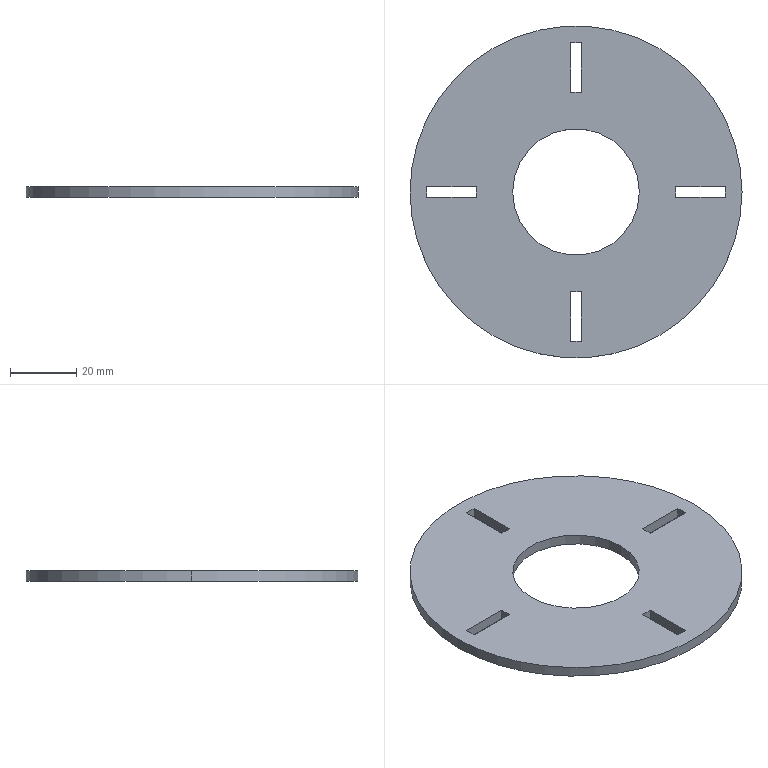Part | SolidWorks | features FlatPattern 1, SMBaseFlange 1, SheetMetal 1 | 1 solid | 22 faces | box 100 x 100 x 3.2 mm | volume 20870 mm3 | plane 18 | cylinder 4 | commonest cylinder face diameters 38.1 x2 100 x2
STEP:
#1=CARTESIAN_POINT('',(-81.781,-15.825,3.2));
#2=VERTEX_POINT('',#1);
#3=CARTESIAN_POINT('',(-43.681,-15.825,3.2));
#4=VERTEX_POINT('',#3);
#5=CARTESIAN_POINT('',(-62.731,-15.825,3.2));
#6=DIRECTION('',(0.,0.,1.));
#7=DIRECTION('',(1.,0.,0.));
#8=AXIS2_PLACEMENT_3D('',#5,#6,#7);
#9=CIRCLE('',#8,19.05);
#10=EDGE_CURVE('',#2,#4,#9,.T.);
#11=ORIENTED_EDGE('',*,*,#10,.T.);
#12=CARTESIAN_POINT('',(-43.681,-15.825,0.));
#13=VERTEX_POINT('',#12);
#14=CARTESIAN_POINT('',(-43.681,-15.825,3.2));
#15=DIRECTION('',(0.,0.,-1.));
#16=VECTOR('',#15,1000.);
#17=LINE('',#14,#16);
#18=EDGE_CURVE('',#4,#13,#17,.T.);
#19=ORIENTED_EDGE('',*,*,#18,.T.);
#20=CARTESIAN_POINT('',(-81.781,-15.825,0.));
#21=VERTEX_POINT('',#20);
#22=CARTESIAN_POINT('',(-62.731,-15.825,0.));
#23=DIRECTION('',(0.,0.,1.));
#24=DIRECTION('',(1.,0.,0.));
#25=AXIS2_PLACEMENT_3D('',#22,#23,#24);
#26=CIRCLE('',#25,19.05);
#27=EDGE_CURVE('',#21,#13,#26,.T.);
#28=ORIENTED_EDGE('',*,*,#27,.F.);
#29=CARTESIAN_POINT('',(-81.781,-15.825,3.2));
#30=DIRECTION('',(0.,0.,-1.));
#31=VECTOR('',#30,1000.);
#32=LINE('',#29,#31);
#33=EDGE_CURVE('',#2,#21,#32,.T.);
#34=ORIENTED_EDGE('',*,*,#33,.F.);
#35=EDGE_LOOP('',(#11,#19,#28,#34));
#36=FACE_OUTER_BOUND('',#35,.T.);
#37=CARTESIAN_POINT('',(-62.731,-15.825,3.2));
#38=DIRECTION('',(0.,0.,-1.));
#39=DIRECTION('',(-1.,0.,0.));
#40=AXIS2_PLACEMENT_3D('',#37,#38,#39);
#41=CYLINDRICAL_SURFACE('',#40,19.05);
#42=ADVANCED_FACE('',(#36),#41,.F.);
#43=CARTESIAN_POINT('',(-12.731,-15.825,3.2));
#44=VERTEX_POINT('',#43);
#45=CARTESIAN_POINT('',(-112.731,-15.825,3.2));
#46=VERTEX_POINT('',#45);
#47=CARTESIAN_POINT('',(-62.731,-15.825,3.2));
#48=DIRECTION('',(0.,0.,1.));
#49=DIRECTION('',(1.,0.,0.));
#50=AXIS2_PLACEMENT_3D('',#47,#48,#49);
#51=CIRCLE('',#50,50.);
#52=EDGE_CURVE('',#44,#46,#51,.T.);
#53=ORIENTED_EDGE('',*,*,#52,.F.);
#54=CARTESIAN_POINT('',(-12.731,-15.825,0.));
#55=VERTEX_POINT('',#54);
#56=CARTESIAN_POINT('',(-12.731,-15.825,3.2));
#57=DIRECTION('',(0.,0.,-1.));
#58=VECTOR('',#57,1000.);
#59=LINE('',#56,#58);
#60=EDGE_CURVE('',#44,#55,#59,.T.);
#61=ORIENTED_EDGE('',*,*,#60,.T.);
#62=CARTESIAN_POINT('',(-112.731,-15.825,0.));
#63=VERTEX_POINT('',#62);
#64=CARTESIAN_POINT('',(-62.731,-15.825,0.));
#65=DIRECTION('',(0.,0.,1.));
#66=DIRECTION('',(1.,0.,0.));
#67=AXIS2_PLACEMENT_3D('',#64,#65,#66);
#68=CIRCLE('',#67,50.);
#69=EDGE_CURVE('',#55,#63,#68,.T.);
#70=ORIENTED_EDGE('',*,*,#69,.T.);
#71=CARTESIAN_POINT('',(-112.731,-15.825,3.2));
#72=DIRECTION('',(0.,0.,-1.));
#73=VECTOR('',#72,1000.);
#74=LINE('',#71,#73);
#75=EDGE_CURVE('',#46,#63,#74,.T.);
#76=ORIENTED_EDGE('',*,*,#75,.F.);
#77=EDGE_LOOP('',(#53,#61,#70,#76));
#78=FACE_OUTER_BOUND('',#77,.T.);
#79=CARTESIAN_POINT('',(-62.731,-15.825,3.2));
#80=DIRECTION('',(0.,0.,-1.));
#81=DIRECTION('',(-1.,0.,0.));
#82=AXIS2_PLACEMENT_3D('',#79,#80,#81);
#83=CYLINDRICAL_SURFACE('',#82,50.);
#84=ADVANCED_FACE('',(#78),#83,.T.);
#85=CARTESIAN_POINT('',(-62.731,-15.825,3.2));
#86=DIRECTION('',(0.,0.,1.));
#87=DIRECTION('',(1.,0.,0.));
#88=AXIS2_PLACEMENT_3D('',#85,#86,#87);
#89=CIRCLE('',#88,50.);
#90=EDGE_CURVE('',#46,#44,#89,.T.);
#91=ORIENTED_EDGE('',*,*,#90,.T.);
#92=ORIENTED_EDGE('',*,*,#52,.T.);
#93=EDGE_LOOP('',(#91,#92));
#94=FACE_OUTER_BOUND('',#93,.T.);
#95=ORIENTED_EDGE('',*,*,#10,.F.);
#96=CARTESIAN_POINT('',(-62.731,-15.825,3.2));
#97=DIRECTION('',(0.,0.,1.));
#98=DIRECTION('',(1.,0.,0.));
#99=AXIS2_PLACEMENT_3D('',#96,#97,#98);
#100=CIRCLE('',#99,19.05);
#101=EDGE_CURVE('',#4,#2,#100,.T.);
#102=ORIENTED_EDGE('',*,*,#101,.F.);
#103=EDGE_LOOP('',(#95,#102));
#104=FACE_BOUND('',#103,.T.);
#105=CARTESIAN_POINT('',(-32.731,-17.425,3.2));
#106=VERTEX_POINT('',#105);
#107=CARTESIAN_POINT('',(-17.731,-17.425,3.2));
#108=VERTEX_POINT('',#107);
#109=CARTESIAN_POINT('',(-32.731,-17.425,3.2));
#110=DIRECTION('',(1.,0.,0.));
#111=VECTOR('',#110,1000.);
#112=LINE('',#109,#111);
#113=EDGE_CURVE('',#106,#108,#112,.T.);
#114=ORIENTED_EDGE('',*,*,#113,.F.);
#115=CARTESIAN_POINT('',(-32.731,-14.225,3.2));
#116=VERTEX_POINT('',#115);
#117=CARTESIAN_POINT('',(-32.731,-14.225,3.2));
#118=DIRECTION('',(0.,-1.,0.));
#119=VECTOR('',#118,1000.);
#120=LINE('',#117,#119);
#121=EDGE_CURVE('',#116,#106,#120,.T.);
#122=ORIENTED_EDGE('',*,*,#121,.F.);
#123=CARTESIAN_POINT('',(-17.731,-14.225,3.2));
#124=VERTEX_POINT('',#123);
#125=CARTESIAN_POINT('',(-32.731,-14.225,3.2));
#126=DIRECTION('',(-1.,0.,0.));
#127=VECTOR('',#126,1000.);
#128=LINE('',#125,#127);
#129=EDGE_CURVE('',#124,#116,#128,.T.);
#130=ORIENTED_EDGE('',*,*,#129,.F.);
#131=CARTESIAN_POINT('',(-17.731,-14.225,3.2));
#132=DIRECTION('',(0.,1.,0.));
#133=VECTOR('',#132,1000.);
#134=LINE('',#131,#133);
#135=EDGE_CURVE('',#108,#124,#134,.T.);
#136=ORIENTED_EDGE('',*,*,#135,.F.);
#137=EDGE_LOOP('',(#114,#122,#130,#136));
#138=FACE_BOUND('',#137,.T.);
#139=CARTESIAN_POINT('',(-64.331,14.175,3.2));
#140=VERTEX_POINT('',#139);
#141=CARTESIAN_POINT('',(-61.131,14.175,3.2));
#142=VERTEX_POINT('',#141);
#143=CARTESIAN_POINT('',(-64.331,14.175,3.2));
#144=DIRECTION('',(1.,0.,0.));
#145=VECTOR('',#144,1000.);
#146=LINE('',#143,#145);
#147=EDGE_CURVE('',#140,#142,#146,.T.);
#148=ORIENTED_EDGE('',*,*,#147,.F.);
#149=CARTESIAN_POINT('',(-64.331,29.175,3.2));
#150=VERTEX_POINT('',#149);
#151=CARTESIAN_POINT('',(-64.331,14.175,3.2));
#152=DIRECTION('',(0.,-1.,0.));
#153=VECTOR('',#152,1000.);
#154=LINE('',#151,#153);
#155=EDGE_CURVE('',#150,#140,#154,.T.);
#156=ORIENTED_EDGE('',*,*,#155,.F.);
#157=CARTESIAN_POINT('',(-61.131,29.175,3.2));
#158=VERTEX_POINT('',#157);
#159=CARTESIAN_POINT('',(-64.331,29.175,3.2));
#160=DIRECTION('',(-1.,0.,0.));
#161=VECTOR('',#160,1000.);
#162=LINE('',#159,#161);
#163=EDGE_CURVE('',#158,#150,#162,.T.);
#164=ORIENTED_EDGE('',*,*,#163,.F.);
#165=CARTESIAN_POINT('',(-61.131,14.175,3.2));
#166=DIRECTION('',(0.,1.,0.));
#167=VECTOR('',#166,1000.);
#168=LINE('',#165,#167);
#169=EDGE_CURVE('',#142,#158,#168,.T.);
#170=ORIENTED_EDGE('',*,*,#169,.F.);
#171=EDGE_LOOP('',(#148,#156,#164,#170));
#172=FACE_BOUND('',#171,.T.);
#173=CARTESIAN_POINT('',(-61.131,-45.825,3.2));
#174=VERTEX_POINT('',#173);
#175=CARTESIAN_POINT('',(-64.331,-45.825,3.2));
#176=VERTEX_POINT('',#175);
#177=CARTESIAN_POINT('',(-61.131,-45.825,3.2));
#178=DIRECTION('',(-1.,0.,0.));
#179=VECTOR('',#178,1000.);
#180=LINE('',#177,#179);
#181=EDGE_CURVE('',#174,#176,#180,.T.);
#182=ORIENTED_EDGE('',*,*,#181,.F.);
#183=CARTESIAN_POINT('',(-61.131,-60.825,3.2));
#184=VERTEX_POINT('',#183);
#185=CARTESIAN_POINT('',(-61.131,-45.825,3.2));
#186=DIRECTION('',(0.,1.,0.));
#187=VECTOR('',#186,1000.);
#188=LINE('',#185,#187);
#189=EDGE_CURVE('',#184,#174,#188,.T.);
#190=ORIENTED_EDGE('',*,*,#189,.F.);
#191=CARTESIAN_POINT('',(-64.331,-60.825,3.2));
#192=VERTEX_POINT('',#191);
#193=CARTESIAN_POINT('',(-61.131,-60.825,3.2));
#194=DIRECTION('',(1.,0.,0.));
#195=VECTOR('',#194,1000.);
#196=LINE('',#193,#195);
#197=EDGE_CURVE('',#192,#184,#196,.T.);
#198=ORIENTED_EDGE('',*,*,#197,.F.);
#199=CARTESIAN_POINT('',(-64.331,-45.825,3.2));
#200=DIRECTION('',(0.,-1.,0.));
#201=VECTOR('',#200,1000.);
#202=LINE('',#199,#201);
#203=EDGE_CURVE('',#176,#192,#202,.T.);
#204=ORIENTED_EDGE('',*,*,#203,.F.);
#205=EDGE_LOOP('',(#182,#190,#198,#204));
#206=FACE_BOUND('',#205,.T.);
#207=CARTESIAN_POINT('',(-92.731,-14.225,3.2));
#208=VERTEX_POINT('',#207);
#209=CARTESIAN_POINT('',(-107.731,-14.225,3.2));
#210=VERTEX_POINT('',#209);
#211=CARTESIAN_POINT('',(-92.731,-14.225,3.2));
#212=DIRECTION('',(-1.,0.,0.));
#213=VECTOR('',#212,1000.);
#214=LINE('',#211,#213);
#215=EDGE_CURVE('',#208,#210,#214,.T.);
#216=ORIENTED_EDGE('',*,*,#215,.F.);
#217=CARTESIAN_POINT('',(-92.731,-17.425,3.2));
#218=VERTEX_POINT('',#217);
#219=CARTESIAN_POINT('',(-92.731,-14.225,3.2));
#220=DIRECTION('',(0.,1.,0.));
#221=VECTOR('',#220,1000.);
#222=LINE('',#219,#221);
#223=EDGE_CURVE('',#218,#208,#222,.T.);
#224=ORIENTED_EDGE('',*,*,#223,.F.);
#225=CARTESIAN_POINT('',(-107.731,-17.425,3.2));
#226=VERTEX_POINT('',#225);
#227=CARTESIAN_POINT('',(-92.731,-17.425,3.2));
#228=DIRECTION('',(1.,0.,0.));
#229=VECTOR('',#228,1000.);
#230=LINE('',#227,#229);
#231=EDGE_CURVE('',#226,#218,#230,.T.);
#232=ORIENTED_EDGE('',*,*,#231,.F.);
#233=CARTESIAN_POINT('',(-107.731,-14.225,3.2));
#234=DIRECTION('',(0.,-1.,0.));
#235=VECTOR('',#234,1000.);
#236=LINE('',#233,#235);
#237=EDGE_CURVE('',#210,#226,#236,.T.);
#238=ORIENTED_EDGE('',*,*,#237,.F.);
#239=EDGE_LOOP('',(#216,#224,#232,#238));
#240=FACE_BOUND('',#239,.T.);
#241=CARTESIAN_POINT('',(-62.731,-15.825,3.2));
#242=DIRECTION('',(0.,0.,1.));
#243=DIRECTION('',(1.,0.,0.));
#244=AXIS2_PLACEMENT_3D('',#241,#242,#243);
#245=PLANE('',#244);
#246=ADVANCED_FACE('',(#94,#104,#138,#172,#206,#240),#245,.T.);
#247=CARTESIAN_POINT('',(-61.131,-60.825,0.));
#248=VERTEX_POINT('',#247);
#249=CARTESIAN_POINT('',(-61.131,-45.825,0.));
#250=VERTEX_POINT('',#249);
#251=CARTESIAN_POINT('',(-61.131,-45.825,0.));
#252=DIRECTION('',(0.,1.,0.));
#253=VECTOR('',#252,1000.);
#254=LINE('',#251,#253);
#255=EDGE_CURVE('',#248,#250,#254,.T.);
#256=ORIENTED_EDGE('',*,*,#255,.T.);
#257=CARTESIAN_POINT('',(-64.331,-45.825,0.));
#258=VERTEX_POINT('',#257);
#259=CARTESIAN_POINT('',(-61.131,-45.825,0.));
#260=DIRECTION('',(-1.,0.,0.));
#261=VECTOR('',#260,1000.);
#262=LINE('',#259,#261);
#263=EDGE_CURVE('',#250,#258,#262,.T.);
#264=ORIENTED_EDGE('',*,*,#263,.T.);
#265=CARTESIAN_POINT('',(-64.331,-60.825,0.));
#266=VERTEX_POINT('',#265);
#267=CARTESIAN_POINT('',(-64.331,-45.825,0.));
#268=DIRECTION('',(0.,-1.,0.));
#269=VECTOR('',#268,1000.);
#270=LINE('',#267,#269);
#271=EDGE_CURVE('',#258,#266,#270,.T.);
#272=ORIENTED_EDGE('',*,*,#271,.T.);
#273=CARTESIAN_POINT('',(-61.131,-60.825,0.));
#274=DIRECTION('',(1.,0.,0.));
#275=VECTOR('',#274,1000.);
#276=LINE('',#273,#275);
#277=EDGE_CURVE('',#266,#248,#276,.T.);
#278=ORIENTED_EDGE('',*,*,#277,.T.);
#279=EDGE_LOOP('',(#256,#264,#272,#278));
#280=FACE_BOUND('',#279,.T.);
#281=CARTESIAN_POINT('',(-32.731,-14.225,0.));
#282=VERTEX_POINT('',#281);
#283=CARTESIAN_POINT('',(-32.731,-17.425,0.));
#284=VERTEX_POINT('',#283);
#285=CARTESIAN_POINT('',(-32.731,-14.225,0.));
#286=DIRECTION('',(0.,-1.,0.));
#287=VECTOR('',#286,1000.);
#288=LINE('',#285,#287);
#289=EDGE_CURVE('',#282,#284,#288,.T.);
#290=ORIENTED_EDGE('',*,*,#289,.T.);
#291=CARTESIAN_POINT('',(-17.731,-17.425,0.));
#292=VERTEX_POINT('',#291);
#293=CARTESIAN_POINT('',(-32.731,-17.425,0.));
#294=DIRECTION('',(1.,0.,0.));
#295=VECTOR('',#294,1000.);
#296=LINE('',#293,#295);
#297=EDGE_CURVE('',#284,#292,#296,.T.);
#298=ORIENTED_EDGE('',*,*,#297,.T.);
#299=CARTESIAN_POINT('',(-17.731,-14.225,0.));
#300=VERTEX_POINT('',#299);
#301=CARTESIAN_POINT('',(-17.731,-14.225,0.));
#302=DIRECTION('',(0.,1.,0.));
#303=VECTOR('',#302,1000.);
#304=LINE('',#301,#303);
#305=EDGE_CURVE('',#292,#300,#304,.T.);
#306=ORIENTED_EDGE('',*,*,#305,.T.);
#307=CARTESIAN_POINT('',(-32.731,-14.225,0.));
#308=DIRECTION('',(-1.,0.,0.));
#309=VECTOR('',#308,1000.);
#310=LINE('',#307,#309);
#311=EDGE_CURVE('',#300,#282,#310,.T.);
#312=ORIENTED_EDGE('',*,*,#311,.T.);
#313=EDGE_LOOP('',(#290,#298,#306,#312));
#314=FACE_BOUND('',#313,.T.);
#315=CARTESIAN_POINT('',(-62.731,-15.825,0.));
#316=DIRECTION('',(0.,0.,1.));
#317=DIRECTION('',(1.,0.,0.));
#318=AXIS2_PLACEMENT_3D('',#315,#316,#317);
#319=CIRCLE('',#318,50.);
#320=EDGE_CURVE('',#63,#55,#319,.T.);
#321=ORIENTED_EDGE('',*,*,#320,.F.);
#322=ORIENTED_EDGE('',*,*,#69,.F.);
#323=EDGE_LOOP('',(#321,#322));
#324=FACE_OUTER_BOUND('',#323,.T.);
#325=ORIENTED_EDGE('',*,*,#27,.T.);
#326=CARTESIAN_POINT('',(-62.731,-15.825,0.));
#327=DIRECTION('',(0.,0.,1.));
#328=DIRECTION('',(1.,0.,0.));
#329=AXIS2_PLACEMENT_3D('',#326,#327,#328);
#330=CIRCLE('',#329,19.05);
#331=EDGE_CURVE('',#13,#21,#330,.T.);
#332=ORIENTED_EDGE('',*,*,#331,.T.);
#333=EDGE_LOOP('',(#325,#332));
#334=FACE_BOUND('',#333,.T.);
#335=CARTESIAN_POINT('',(-64.331,29.175,0.));
#336=VERTEX_POINT('',#335);
#337=CARTESIAN_POINT('',(-64.331,14.175,0.));
#338=VERTEX_POINT('',#337);
#339=CARTESIAN_POINT('',(-64.331,14.175,0.));
#340=DIRECTION('',(0.,-1.,0.));
#341=VECTOR('',#340,1000.);
#342=LINE('',#339,#341);
#343=EDGE_CURVE('',#336,#338,#342,.T.);
#344=ORIENTED_EDGE('',*,*,#343,.T.);
#345=CARTESIAN_POINT('',(-61.131,14.175,0.));
#346=VERTEX_POINT('',#345);
#347=CARTESIAN_POINT('',(-64.331,14.175,0.));
#348=DIRECTION('',(1.,0.,0.));
#349=VECTOR('',#348,1000.);
#350=LINE('',#347,#349);
#351=EDGE_CURVE('',#338,#346,#350,.T.);
#352=ORIENTED_EDGE('',*,*,#351,.T.);
#353=CARTESIAN_POINT('',(-61.131,29.175,0.));
#354=VERTEX_POINT('',#353);
#355=CARTESIAN_POINT('',(-61.131,14.175,0.));
#356=DIRECTION('',(0.,1.,0.));
#357=VECTOR('',#356,1000.);
#358=LINE('',#355,#357);
#359=EDGE_CURVE('',#346,#354,#358,.T.);
#360=ORIENTED_EDGE('',*,*,#359,.T.);
#361=CARTESIAN_POINT('',(-64.331,29.175,0.));
#362=DIRECTION('',(-1.,0.,0.));
#363=VECTOR('',#362,1000.);
#364=LINE('',#361,#363);
#365=EDGE_CURVE('',#354,#336,#364,.T.);
#366=ORIENTED_EDGE('',*,*,#365,.T.);
#367=EDGE_LOOP('',(#344,#352,#360,#366));
#368=FACE_BOUND('',#367,.T.);
#369=CARTESIAN_POINT('',(-92.731,-17.425,0.));
#370=VERTEX_POINT('',#369);
#371=CARTESIAN_POINT('',(-92.731,-14.225,0.));
#372=VERTEX_POINT('',#371);
#373=CARTESIAN_POINT('',(-92.731,-14.225,0.));
#374=DIRECTION('',(0.,1.,0.));
#375=VECTOR('',#374,1000.);
#376=LINE('',#373,#375);
#377=EDGE_CURVE('',#370,#372,#376,.T.);
#378=ORIENTED_EDGE('',*,*,#377,.T.);
#379=CARTESIAN_POINT('',(-107.731,-14.225,0.));
#380=VERTEX_POINT('',#379);
#381=CARTESIAN_POINT('',(-92.731,-14.225,0.));
#382=DIRECTION('',(-1.,0.,0.));
#383=VECTOR('',#382,1000.);
#384=LINE('',#381,#383);
#385=EDGE_CURVE('',#372,#380,#384,.T.);
#386=ORIENTED_EDGE('',*,*,#385,.T.);
#387=CARTESIAN_POINT('',(-107.731,-17.425,0.));
#388=VERTEX_POINT('',#387);
#389=CARTESIAN_POINT('',(-107.731,-14.225,0.));
#390=DIRECTION('',(0.,-1.,0.));
#391=VECTOR('',#390,1000.);
#392=LINE('',#389,#391);
#393=EDGE_CURVE('',#380,#388,#392,.T.);
#394=ORIENTED_EDGE('',*,*,#393,.T.);
#395=CARTESIAN_POINT('',(-92.731,-17.425,0.));
#396=DIRECTION('',(1.,0.,0.));
#397=VECTOR('',#396,1000.);
#398=LINE('',#395,#397);
#399=EDGE_CURVE('',#388,#370,#398,.T.);
#400=ORIENTED_EDGE('',*,*,#399,.T.);
#401=EDGE_LOOP('',(#378,#386,#394,#400));
#402=FACE_BOUND('',#401,.T.);
#403=CARTESIAN_POINT('',(-62.731,-15.825,0.));
#404=DIRECTION('',(0.,0.,1.));
#405=DIRECTION('',(1.,0.,0.));
#406=AXIS2_PLACEMENT_3D('',#403,#404,#405);
#407=PLANE('',#406);
#408=ADVANCED_FACE('',(#280,#314,#324,#334,#368,#402),#407,.F.);
#409=ORIENTED_EDGE('',*,*,#60,.F.);
#410=ORIENTED_EDGE('',*,*,#90,.F.);
#411=ORIENTED_EDGE('',*,*,#75,.T.);
#412=ORIENTED_EDGE('',*,*,#320,.T.);
#413=EDGE_LOOP('',(#409,#410,#411,#412));
#414=FACE_OUTER_BOUND('',#413,.T.);
#415=CARTESIAN_POINT('',(-62.731,-15.825,3.2));
#416=DIRECTION('',(0.,0.,-1.));
#417=DIRECTION('',(-1.,0.,0.));
#418=AXIS2_PLACEMENT_3D('',#415,#416,#417);
#419=CYLINDRICAL_SURFACE('',#418,50.);
#420=ADVANCED_FACE('',(#414),#419,.T.);
#421=ORIENTED_EDGE('',*,*,#18,.F.);
#422=ORIENTED_EDGE('',*,*,#101,.T.);
#423=ORIENTED_EDGE('',*,*,#33,.T.);
#424=ORIENTED_EDGE('',*,*,#331,.F.);
#425=EDGE_LOOP('',(#421,#422,#423,#424));
#426=FACE_OUTER_BOUND('',#425,.T.);
#427=CARTESIAN_POINT('',(-62.731,-15.825,3.2));
#428=DIRECTION('',(0.,0.,-1.));
#429=DIRECTION('',(-1.,0.,0.));
#430=AXIS2_PLACEMENT_3D('',#427,#428,#429);
#431=CYLINDRICAL_SURFACE('',#430,19.05);
#432=ADVANCED_FACE('',(#426),#431,.F.);
#433=ORIENTED_EDGE('',*,*,#289,.F.);
#434=CARTESIAN_POINT('',(-32.731,-14.225,3.2));
#435=DIRECTION('',(0.,0.,-1.));
#436=VECTOR('',#435,1000.);
#437=LINE('',#434,#436);
#438=EDGE_CURVE('',#116,#282,#437,.T.);
#439=ORIENTED_EDGE('',*,*,#438,.F.);
#440=ORIENTED_EDGE('',*,*,#121,.T.);
#441=CARTESIAN_POINT('',(-32.731,-17.425,3.2));
#442=DIRECTION('',(0.,0.,-1.));
#443=VECTOR('',#442,1000.);
#444=LINE('',#441,#443);
#445=EDGE_CURVE('',#106,#284,#444,.T.);
#446=ORIENTED_EDGE('',*,*,#445,.T.);
#447=EDGE_LOOP('',(#433,#439,#440,#446));
#448=FACE_OUTER_BOUND('',#447,.T.);
#449=CARTESIAN_POINT('',(-32.731,-14.225,3.2));
#450=DIRECTION('',(1.,0.,0.));
#451=DIRECTION('',(0.,0.,-1.));
#452=AXIS2_PLACEMENT_3D('',#449,#450,#451);
#453=PLANE('',#452);
#454=ADVANCED_FACE('',(#448),#453,.T.);
#455=ORIENTED_EDGE('',*,*,#297,.F.);
#456=ORIENTED_EDGE('',*,*,#445,.F.);
#457=ORIENTED_EDGE('',*,*,#113,.T.);
#458=CARTESIAN_POINT('',(-17.731,-17.425,3.2));
#459=DIRECTION('',(0.,0.,-1.));
#460=VECTOR('',#459,1000.);
#461=LINE('',#458,#460);
#462=EDGE_CURVE('',#108,#292,#461,.T.);
#463=ORIENTED_EDGE('',*,*,#462,.T.);
#464=EDGE_LOOP('',(#455,#456,#457,#463));
#465=FACE_OUTER_BOUND('',#464,.T.);
#466=CARTESIAN_POINT('',(-32.731,-17.425,3.2));
#467=DIRECTION('',(0.,1.,0.));
#468=DIRECTION('',(0.,0.,1.));
#469=AXIS2_PLACEMENT_3D('',#466,#467,#468);
#470=PLANE('',#469);
#471=ADVANCED_FACE('',(#465),#470,.T.);
#472=ORIENTED_EDGE('',*,*,#305,.F.);
#473=ORIENTED_EDGE('',*,*,#462,.F.);
#474=ORIENTED_EDGE('',*,*,#135,.T.);
#475=CARTESIAN_POINT('',(-17.731,-14.225,3.2));
#476=DIRECTION('',(0.,0.,-1.));
#477=VECTOR('',#476,1000.);
#478=LINE('',#475,#477);
#479=EDGE_CURVE('',#124,#300,#478,.T.);
#480=ORIENTED_EDGE('',*,*,#479,.T.);
#481=EDGE_LOOP('',(#472,#473,#474,#480));
#482=FACE_OUTER_BOUND('',#481,.T.);
#483=CARTESIAN_POINT('',(-17.731,-14.225,3.2));
#484=DIRECTION('',(-1.,0.,0.));
#485=DIRECTION('',(0.,0.,1.));
#486=AXIS2_PLACEMENT_3D('',#483,#484,#485);
#487=PLANE('',#486);
#488=ADVANCED_FACE('',(#482),#487,.T.);
#489=ORIENTED_EDGE('',*,*,#311,.F.);
#490=ORIENTED_EDGE('',*,*,#479,.F.);
#491=ORIENTED_EDGE('',*,*,#129,.T.);
#492=ORIENTED_EDGE('',*,*,#438,.T.);
#493=EDGE_LOOP('',(#489,#490,#491,#492));
#494=FACE_OUTER_BOUND('',#493,.T.);
#495=CARTESIAN_POINT('',(-32.731,-14.225,3.2));
#496=DIRECTION('',(0.,-1.,0.));
#497=DIRECTION('',(0.,0.,-1.));
#498=AXIS2_PLACEMENT_3D('',#495,#496,#497);
#499=PLANE('',#498);
#500=ADVANCED_FACE('',(#494),#499,.T.);
#501=ORIENTED_EDGE('',*,*,#343,.F.);
#502=CARTESIAN_POINT('',(-64.331,29.175,3.2));
#503=DIRECTION('',(0.,0.,-1.));
#504=VECTOR('',#503,1000.);
#505=LINE('',#502,#504);
#506=EDGE_CURVE('',#150,#336,#505,.T.);
#507=ORIENTED_EDGE('',*,*,#506,.F.);
#508=ORIENTED_EDGE('',*,*,#155,.T.);
#509=CARTESIAN_POINT('',(-64.331,14.175,3.2));
#510=DIRECTION('',(0.,0.,-1.));
#511=VECTOR('',#510,1000.);
#512=LINE('',#509,#511);
#513=EDGE_CURVE('',#140,#338,#512,.T.);
#514=ORIENTED_EDGE('',*,*,#513,.T.);
#515=EDGE_LOOP('',(#501,#507,#508,#514));
#516=FACE_OUTER_BOUND('',#515,.T.);
#517=CARTESIAN_POINT('',(-64.331,14.175,3.2));
#518=DIRECTION('',(1.,0.,0.));
#519=DIRECTION('',(0.,0.,-1.));
#520=AXIS2_PLACEMENT_3D('',#517,#518,#519);
#521=PLANE('',#520);
#522=ADVANCED_FACE('',(#516),#521,.T.);
#523=ORIENTED_EDGE('',*,*,#351,.F.);
#524=ORIENTED_EDGE('',*,*,#513,.F.);
#525=ORIENTED_EDGE('',*,*,#147,.T.);
#526=CARTESIAN_POINT('',(-61.131,14.175,3.2));
#527=DIRECTION('',(0.,0.,-1.));
#528=VECTOR('',#527,1000.);
#529=LINE('',#526,#528);
#530=EDGE_CURVE('',#142,#346,#529,.T.);
#531=ORIENTED_EDGE('',*,*,#530,.T.);
#532=EDGE_LOOP('',(#523,#524,#525,#531));
#533=FACE_OUTER_BOUND('',#532,.T.);
#534=CARTESIAN_POINT('',(-64.331,14.175,3.2));
#535=DIRECTION('',(0.,1.,0.));
#536=DIRECTION('',(0.,0.,1.));
#537=AXIS2_PLACEMENT_3D('',#534,#535,#536);
#538=PLANE('',#537);
#539=ADVANCED_FACE('',(#533),#538,.T.);
#540=ORIENTED_EDGE('',*,*,#359,.F.);
#541=ORIENTED_EDGE('',*,*,#530,.F.);
#542=ORIENTED_EDGE('',*,*,#169,.T.);
#543=CARTESIAN_POINT('',(-61.131,29.175,3.2));
#544=DIRECTION('',(0.,0.,-1.));
#545=VECTOR('',#544,1000.);
#546=LINE('',#543,#545);
#547=EDGE_CURVE('',#158,#354,#546,.T.);
#548=ORIENTED_EDGE('',*,*,#547,.T.);
#549=EDGE_LOOP('',(#540,#541,#542,#548));
#550=FACE_OUTER_BOUND('',#549,.T.);
#551=CARTESIAN_POINT('',(-61.131,14.175,3.2));
#552=DIRECTION('',(-1.,0.,0.));
#553=DIRECTION('',(0.,0.,1.));
#554=AXIS2_PLACEMENT_3D('',#551,#552,#553);
#555=PLANE('',#554);
#556=ADVANCED_FACE('',(#550),#555,.T.);
#557=ORIENTED_EDGE('',*,*,#365,.F.);
#558=ORIENTED_EDGE('',*,*,#547,.F.);
#559=ORIENTED_EDGE('',*,*,#163,.T.);
#560=ORIENTED_EDGE('',*,*,#506,.T.);
#561=EDGE_LOOP('',(#557,#558,#559,#560));
#562=FACE_OUTER_BOUND('',#561,.T.);
#563=CARTESIAN_POINT('',(-64.331,29.175,3.2));
#564=DIRECTION('',(0.,-1.,0.));
#565=DIRECTION('',(0.,0.,-1.));
#566=AXIS2_PLACEMENT_3D('',#563,#564,#565);
#567=PLANE('',#566);
#568=ADVANCED_FACE('',(#562),#567,.T.);
#569=ORIENTED_EDGE('',*,*,#255,.F.);
#570=CARTESIAN_POINT('',(-61.131,-60.825,3.2));
#571=DIRECTION('',(0.,0.,-1.));
#572=VECTOR('',#571,1000.);
#573=LINE('',#570,#572);
#574=EDGE_CURVE('',#184,#248,#573,.T.);
#575=ORIENTED_EDGE('',*,*,#574,.F.);
#576=ORIENTED_EDGE('',*,*,#189,.T.);
#577=CARTESIAN_POINT('',(-61.131,-45.825,3.2));
#578=DIRECTION('',(0.,0.,-1.));
#579=VECTOR('',#578,1000.);
#580=LINE('',#577,#579);
#581=EDGE_CURVE('',#174,#250,#580,.T.);
#582=ORIENTED_EDGE('',*,*,#581,.T.);
#583=EDGE_LOOP('',(#569,#575,#576,#582));
#584=FACE_OUTER_BOUND('',#583,.T.);
#585=CARTESIAN_POINT('',(-61.131,-45.825,3.2));
#586=DIRECTION('',(-1.,0.,0.));
#587=DIRECTION('',(0.,-1.,0.));
#588=AXIS2_PLACEMENT_3D('',#585,#586,#587);
#589=PLANE('',#588);
#590=ADVANCED_FACE('',(#584),#589,.T.);
#591=ORIENTED_EDGE('',*,*,#263,.F.);
#592=ORIENTED_EDGE('',*,*,#581,.F.);
#593=ORIENTED_EDGE('',*,*,#181,.T.);
#594=CARTESIAN_POINT('',(-64.331,-45.825,3.2));
#595=DIRECTION('',(0.,0.,-1.));
#596=VECTOR('',#595,1000.);
#597=LINE('',#594,#596);
#598=EDGE_CURVE('',#176,#258,#597,.T.);
#599=ORIENTED_EDGE('',*,*,#598,.T.);
#600=EDGE_LOOP('',(#591,#592,#593,#599));
#601=FACE_OUTER_BOUND('',#600,.T.);
#602=CARTESIAN_POINT('',(-61.131,-45.825,3.2));
#603=DIRECTION('',(0.,-1.,0.));
#604=DIRECTION('',(0.,0.,-1.));
#605=AXIS2_PLACEMENT_3D('',#602,#603,#604);
#606=PLANE('',#605);
#607=ADVANCED_FACE('',(#601),#606,.T.);
#608=ORIENTED_EDGE('',*,*,#271,.F.);
#609=ORIENTED_EDGE('',*,*,#598,.F.);
#610=ORIENTED_EDGE('',*,*,#203,.T.);
#611=CARTESIAN_POINT('',(-64.331,-60.825,3.2));
#612=DIRECTION('',(0.,0.,-1.));
#613=VECTOR('',#612,1000.);
#614=LINE('',#611,#613);
#615=EDGE_CURVE('',#192,#266,#614,.T.);
#616=ORIENTED_EDGE('',*,*,#615,.T.);
#617=EDGE_LOOP('',(#608,#609,#610,#616));
#618=FACE_OUTER_BOUND('',#617,.T.);
#619=CARTESIAN_POINT('',(-64.331,-45.825,3.2));
#620=DIRECTION('',(1.,0.,0.));
#621=DIRECTION('',(0.,1.,0.));
#622=AXIS2_PLACEMENT_3D('',#619,#620,#621);
#623=PLANE('',#622);
#624=ADVANCED_FACE('',(#618),#623,.T.);
#625=ORIENTED_EDGE('',*,*,#277,.F.);
#626=ORIENTED_EDGE('',*,*,#615,.F.);
#627=ORIENTED_EDGE('',*,*,#197,.T.);
#628=ORIENTED_EDGE('',*,*,#574,.T.);
#629=EDGE_LOOP('',(#625,#626,#627,#628));
#630=FACE_OUTER_BOUND('',#629,.T.);
#631=CARTESIAN_POINT('',(-61.131,-60.825,3.2));
#632=DIRECTION('',(0.,1.,0.));
#633=DIRECTION('',(0.,0.,1.));
#634=AXIS2_PLACEMENT_3D('',#631,#632,#633);
#635=PLANE('',#634);
#636=ADVANCED_FACE('',(#630),#635,.T.);
#637=ORIENTED_EDGE('',*,*,#377,.F.);
#638=CARTESIAN_POINT('',(-92.731,-17.425,3.2));
#639=DIRECTION('',(0.,0.,-1.));
#640=VECTOR('',#639,1000.);
#641=LINE('',#638,#640);
#642=EDGE_CURVE('',#218,#370,#641,.T.);
#643=ORIENTED_EDGE('',*,*,#642,.F.);
#644=ORIENTED_EDGE('',*,*,#223,.T.);
#645=CARTESIAN_POINT('',(-92.731,-14.225,3.2));
#646=DIRECTION('',(0.,0.,-1.));
#647=VECTOR('',#646,1000.);
#648=LINE('',#645,#647);
#649=EDGE_CURVE('',#208,#372,#648,.T.);
#650=ORIENTED_EDGE('',*,*,#649,.T.);
#651=EDGE_LOOP('',(#637,#643,#644,#650));
#652=FACE_OUTER_BOUND('',#651,.T.);
#653=CARTESIAN_POINT('',(-92.731,-14.225,3.2));
#654=DIRECTION('',(-1.,0.,0.));
#655=DIRECTION('',(0.,0.,1.));
#656=AXIS2_PLACEMENT_3D('',#653,#654,#655);
#657=PLANE('',#656);
#658=ADVANCED_FACE('',(#652),#657,.T.);
#659=ORIENTED_EDGE('',*,*,#385,.F.);
#660=ORIENTED_EDGE('',*,*,#649,.F.);
#661=ORIENTED_EDGE('',*,*,#215,.T.);
#662=CARTESIAN_POINT('',(-107.731,-14.225,3.2));
#663=DIRECTION('',(0.,0.,-1.));
#664=VECTOR('',#663,1000.);
#665=LINE('',#662,#664);
#666=EDGE_CURVE('',#210,#380,#665,.T.);
#667=ORIENTED_EDGE('',*,*,#666,.T.);
#668=EDGE_LOOP('',(#659,#660,#661,#667));
#669=FACE_OUTER_BOUND('',#668,.T.);
#670=CARTESIAN_POINT('',(-92.731,-14.225,3.2));
#671=DIRECTION('',(0.,-1.,0.));
#672=DIRECTION('',(1.,0.,0.));
#673=AXIS2_PLACEMENT_3D('',#670,#671,#672);
#674=PLANE('',#673);
#675=ADVANCED_FACE('',(#669),#674,.T.);
#676=ORIENTED_EDGE('',*,*,#393,.F.);
#677=ORIENTED_EDGE('',*,*,#666,.F.);
#678=ORIENTED_EDGE('',*,*,#237,.T.);
#679=CARTESIAN_POINT('',(-107.731,-17.425,3.2));
#680=DIRECTION('',(0.,0.,-1.));
#681=VECTOR('',#680,1000.);
#682=LINE('',#679,#681);
#683=EDGE_CURVE('',#226,#388,#682,.T.);
#684=ORIENTED_EDGE('',*,*,#683,.T.);
#685=EDGE_LOOP('',(#676,#677,#678,#684));
#686=FACE_OUTER_BOUND('',#685,.T.);
#687=CARTESIAN_POINT('',(-107.731,-14.225,3.2));
#688=DIRECTION('',(1.,0.,0.));
#689=DIRECTION('',(0.,0.,-1.));
#690=AXIS2_PLACEMENT_3D('',#687,#688,#689);
#691=PLANE('',#690);
#692=ADVANCED_FACE('',(#686),#691,.T.);
#693=ORIENTED_EDGE('',*,*,#399,.F.);
#694=ORIENTED_EDGE('',*,*,#683,.F.);
#695=ORIENTED_EDGE('',*,*,#231,.T.);
#696=ORIENTED_EDGE('',*,*,#642,.T.);
#697=EDGE_LOOP('',(#693,#694,#695,#696));
#698=FACE_OUTER_BOUND('',#697,.T.);
#699=CARTESIAN_POINT('',(-92.731,-17.425,3.2));
#700=DIRECTION('',(0.,1.,0.));
#701=DIRECTION('',(-1.,0.,0.));
#702=AXIS2_PLACEMENT_3D('',#699,#700,#701);
#703=PLANE('',#702);
#704=ADVANCED_FACE('',(#698),#703,.T.);
#705=CLOSED_SHELL('',(#42,#84,#246,#408,#420,#432,#454,#471,#488,#500,#522,#539,#556,#568,#590,#607,#624,#636,#658,#675,#692,#704));
#706=MANIFOLD_SOLID_BREP('',#705);
#707=CARTESIAN_POINT('',(0.,0.,0.));
#708=DIRECTION('',(0.,0.,1.));
#709=DIRECTION('',(1.,0.,0.));
#710=AXIS2_PLACEMENT_3D('',#707,#708,#709);
#711=(LENGTH_UNIT()NAMED_UNIT(*)SI_UNIT(.MILLI.,.METRE.));
#712=UNCERTAINTY_MEASURE_WITH_UNIT(LENGTH_MEASURE(0.00001),#711,'','');
#713=(NAMED_UNIT(*)PLANE_ANGLE_UNIT()SI_UNIT($,.RADIAN.));
#714=(NAMED_UNIT(*)SI_UNIT($,.STERADIAN.)SOLID_ANGLE_UNIT());
#715=(GEOMETRIC_REPRESENTATION_CONTEXT(3)GLOBAL_UNCERTAINTY_ASSIGNED_CONTEXT((#712))GLOBAL_UNIT_ASSIGNED_CONTEXT((#711,#713,#714))REPRESENTATION_CONTEXT('',''));
#716=ADVANCED_BREP_SHAPE_REPRESENTATION('',(#706,#710),#715);